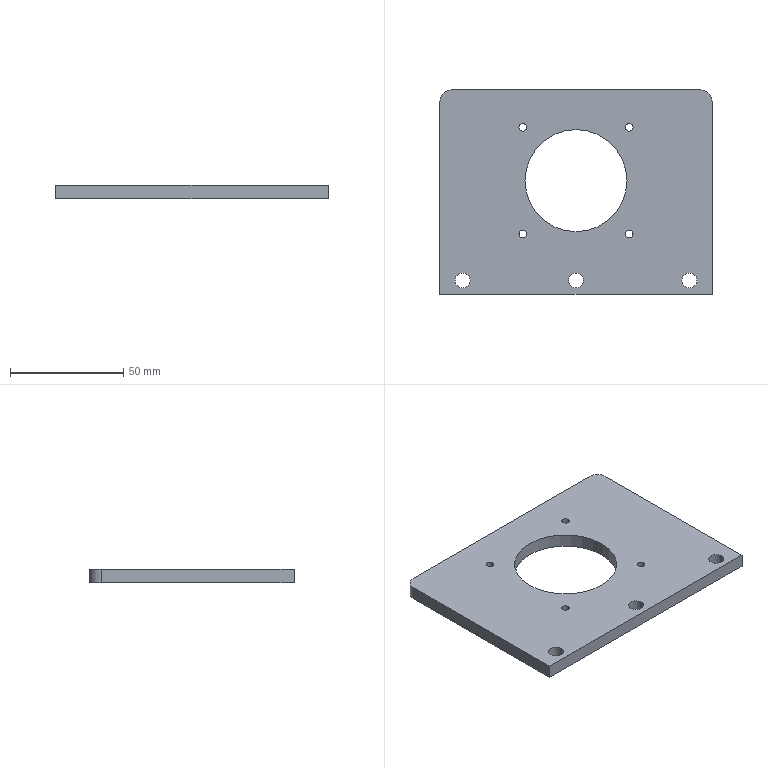Part | STEP file | PN_0022 | 1 solid | 24 faces | box 120 x 90 x 6 mm | volume 54372 mm3 | cylinder 18 | plane 6 | commonest cylinder face diameters 3.3 x8 6.6 x6 10 x2 45 x2